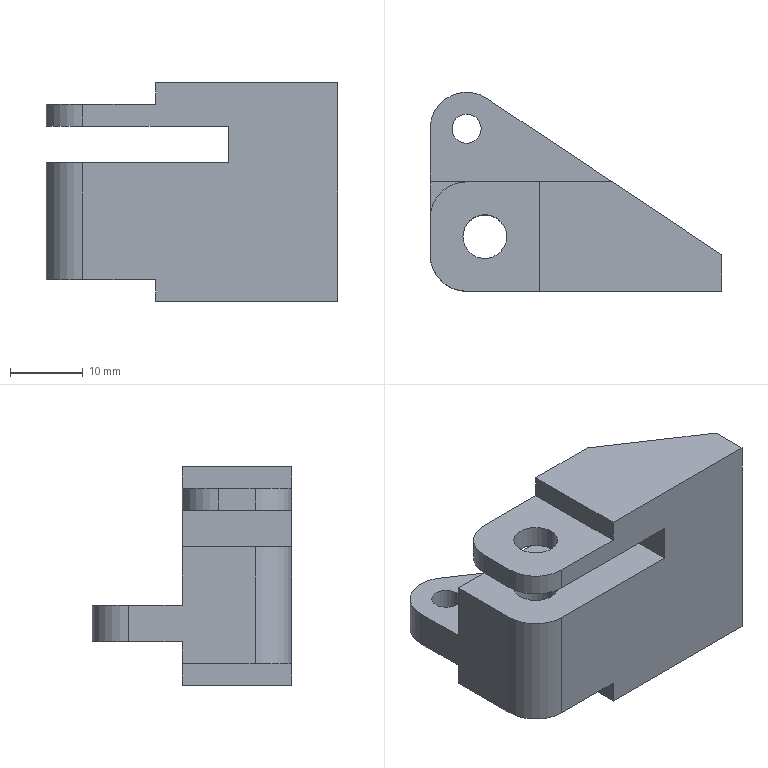Part | SolidWorks | features ICE 4, Fillet 2, Extrusion 1 | 1 solid | 29 faces | box 40 x 27.324 x 30 mm | volume 12750 mm3 | plane 19 | cylinder 10 | commonest cylinder face diameters 6 x4 10 x4 4 x2
STEP:
#1=CARTESIAN_POINT('',(-35.5,7.5,-12.));
#2=VERTEX_POINT('',#1);
#3=CARTESIAN_POINT('',(-29.5,7.5,-12.));
#4=VERTEX_POINT('',#3);
#5=CARTESIAN_POINT('',(-32.5,7.5,-12.));
#6=DIRECTION('',(0.,0.,1.));
#7=DIRECTION('',(1.,0.,0.));
#8=AXIS2_PLACEMENT_3D('',#5,#6,#7);
#9=CIRCLE('',#8,3.);
#10=EDGE_CURVE('',#2,#4,#9,.T.);
#11=ORIENTED_EDGE('',*,*,#10,.F.);
#12=CARTESIAN_POINT('',(-35.5,7.5,4.));
#13=VERTEX_POINT('',#12);
#14=CARTESIAN_POINT('',(-35.5,7.5,-15.));
#15=DIRECTION('',(0.,0.,1.));
#16=VECTOR('',#15,1000.);
#17=LINE('',#14,#16);
#18=EDGE_CURVE('',#2,#13,#17,.T.);
#19=ORIENTED_EDGE('',*,*,#18,.T.);
#20=CARTESIAN_POINT('',(-29.5,7.5,4.));
#21=VERTEX_POINT('',#20);
#22=CARTESIAN_POINT('',(-32.5,7.5,4.));
#23=DIRECTION('',(0.,0.,-1.));
#24=DIRECTION('',(-1.,0.,0.));
#25=AXIS2_PLACEMENT_3D('',#22,#23,#24);
#26=CIRCLE('',#25,3.);
#27=EDGE_CURVE('',#21,#13,#26,.T.);
#28=ORIENTED_EDGE('',*,*,#27,.F.);
#29=CARTESIAN_POINT('',(-29.5,7.5,-15.));
#30=DIRECTION('',(0.,0.,1.));
#31=VECTOR('',#30,1000.);
#32=LINE('',#29,#31);
#33=EDGE_CURVE('',#4,#21,#32,.T.);
#34=ORIENTED_EDGE('',*,*,#33,.F.);
#35=EDGE_LOOP('',(#11,#19,#28,#34));
#36=FACE_OUTER_BOUND('',#35,.T.);
#37=CARTESIAN_POINT('',(-32.5,7.5,-15.));
#38=DIRECTION('',(0.,0.,1.));
#39=DIRECTION('',(1.,0.,0.));
#40=AXIS2_PLACEMENT_3D('',#37,#38,#39);
#41=CYLINDRICAL_SURFACE('',#40,3.);
#42=ADVANCED_FACE('',(#36),#41,.F.);
#43=CARTESIAN_POINT('',(-35.5,7.5,9.));
#44=VERTEX_POINT('',#43);
#45=CARTESIAN_POINT('',(-29.5,7.5,9.));
#46=VERTEX_POINT('',#45);
#47=CARTESIAN_POINT('',(-32.5,7.5,9.));
#48=DIRECTION('',(0.,0.,1.));
#49=DIRECTION('',(1.,0.,0.));
#50=AXIS2_PLACEMENT_3D('',#47,#48,#49);
#51=CIRCLE('',#50,3.);
#52=EDGE_CURVE('',#44,#46,#51,.T.);
#53=ORIENTED_EDGE('',*,*,#52,.F.);
#54=CARTESIAN_POINT('',(-35.5,7.5,12.));
#55=VERTEX_POINT('',#54);
#56=CARTESIAN_POINT('',(-35.5,7.5,-15.));
#57=DIRECTION('',(0.,0.,1.));
#58=VECTOR('',#57,1000.);
#59=LINE('',#56,#58);
#60=EDGE_CURVE('',#44,#55,#59,.T.);
#61=ORIENTED_EDGE('',*,*,#60,.T.);
#62=CARTESIAN_POINT('',(-29.5,7.5,12.));
#63=VERTEX_POINT('',#62);
#64=CARTESIAN_POINT('',(-32.5,7.5,12.));
#65=DIRECTION('',(0.,0.,1.));
#66=DIRECTION('',(1.,0.,0.));
#67=AXIS2_PLACEMENT_3D('',#64,#65,#66);
#68=CIRCLE('',#67,3.);
#69=EDGE_CURVE('',#55,#63,#68,.T.);
#70=ORIENTED_EDGE('',*,*,#69,.T.);
#71=CARTESIAN_POINT('',(-29.5,7.5,-15.));
#72=DIRECTION('',(0.,0.,1.));
#73=VECTOR('',#72,1000.);
#74=LINE('',#71,#73);
#75=EDGE_CURVE('',#46,#63,#74,.T.);
#76=ORIENTED_EDGE('',*,*,#75,.F.);
#77=EDGE_LOOP('',(#53,#61,#70,#76));
#78=FACE_OUTER_BOUND('',#77,.T.);
#79=CARTESIAN_POINT('',(-32.5,7.5,-15.));
#80=DIRECTION('',(0.,0.,1.));
#81=DIRECTION('',(1.,0.,0.));
#82=AXIS2_PLACEMENT_3D('',#79,#80,#81);
#83=CYLINDRICAL_SURFACE('',#82,3.);
#84=ADVANCED_FACE('',(#78),#83,.F.);
#85=CARTESIAN_POINT('',(-37.,22.324,-4.));
#86=VERTEX_POINT('',#85);
#87=CARTESIAN_POINT('',(-33.,22.324,-4.));
#88=VERTEX_POINT('',#87);
#89=CARTESIAN_POINT('',(-35.,22.324,-4.));
#90=DIRECTION('',(0.,0.,1.));
#91=DIRECTION('',(1.,0.,0.));
#92=AXIS2_PLACEMENT_3D('',#89,#90,#91);
#93=CIRCLE('',#92,2.);
#94=EDGE_CURVE('',#86,#88,#93,.T.);
#95=ORIENTED_EDGE('',*,*,#94,.T.);
#96=CARTESIAN_POINT('',(-33.,22.324,-9.));
#97=VERTEX_POINT('',#96);
#98=CARTESIAN_POINT('',(-33.,22.324,-4.));
#99=DIRECTION('',(0.,0.,-1.));
#100=VECTOR('',#99,1000.);
#101=LINE('',#98,#100);
#102=EDGE_CURVE('',#88,#97,#101,.T.);
#103=ORIENTED_EDGE('',*,*,#102,.T.);
#104=CARTESIAN_POINT('',(-37.,22.324,-9.));
#105=VERTEX_POINT('',#104);
#106=CARTESIAN_POINT('',(-35.,22.324,-9.));
#107=DIRECTION('',(0.,0.,1.));
#108=DIRECTION('',(1.,0.,0.));
#109=AXIS2_PLACEMENT_3D('',#106,#107,#108);
#110=CIRCLE('',#109,2.);
#111=EDGE_CURVE('',#105,#97,#110,.T.);
#112=ORIENTED_EDGE('',*,*,#111,.F.);
#113=CARTESIAN_POINT('',(-37.,22.324,-4.));
#114=DIRECTION('',(0.,0.,-1.));
#115=VECTOR('',#114,1000.);
#116=LINE('',#113,#115);
#117=EDGE_CURVE('',#86,#105,#116,.T.);
#118=ORIENTED_EDGE('',*,*,#117,.F.);
#119=EDGE_LOOP('',(#95,#103,#112,#118));
#120=FACE_OUTER_BOUND('',#119,.T.);
#121=CARTESIAN_POINT('',(-35.,22.324,-4.));
#122=DIRECTION('',(0.,0.,-1.));
#123=DIRECTION('',(-1.,0.,0.));
#124=AXIS2_PLACEMENT_3D('',#121,#122,#123);
#125=CYLINDRICAL_SURFACE('',#124,2.);
#126=ADVANCED_FACE('',(#120),#125,.F.);
#127=CARTESIAN_POINT('',(-40.,15.,-9.));
#128=VERTEX_POINT('',#127);
#129=CARTESIAN_POINT('',(-15.,15.,-9.));
#130=VERTEX_POINT('',#129);
#131=CARTESIAN_POINT('',(-40.,15.,-9.));
#132=DIRECTION('',(1.,0.,0.));
#133=VECTOR('',#132,1000.);
#134=LINE('',#131,#133);
#135=EDGE_CURVE('',#128,#130,#134,.T.);
#136=ORIENTED_EDGE('',*,*,#135,.T.);
#137=CARTESIAN_POINT('',(-15.,15.,-15.));
#138=VERTEX_POINT('',#137);
#139=CARTESIAN_POINT('',(-15.,15.,15.));
#140=DIRECTION('',(0.,0.,-1.));
#141=VECTOR('',#140,1000.);
#142=LINE('',#139,#141);
#143=EDGE_CURVE('',#130,#138,#142,.T.);
#144=ORIENTED_EDGE('',*,*,#143,.T.);
#145=CARTESIAN_POINT('',(-25.,15.,-15.));
#146=VERTEX_POINT('',#145);
#147=CARTESIAN_POINT('',(-15.,15.,-15.));
#148=DIRECTION('',(-1.,0.,0.));
#149=VECTOR('',#148,1000.);
#150=LINE('',#147,#149);
#151=EDGE_CURVE('',#138,#146,#150,.T.);
#152=ORIENTED_EDGE('',*,*,#151,.T.);
#153=CARTESIAN_POINT('',(-25.,15.,-12.));
#154=VERTEX_POINT('',#153);
#155=CARTESIAN_POINT('',(-25.,15.,-32.358));
#156=DIRECTION('',(0.,0.,-1.));
#157=VECTOR('',#156,1000.);
#158=LINE('',#155,#157);
#159=EDGE_CURVE('',#154,#146,#158,.T.);
#160=ORIENTED_EDGE('',*,*,#159,.F.);
#161=CARTESIAN_POINT('',(-40.,15.,-12.));
#162=VERTEX_POINT('',#161);
#163=CARTESIAN_POINT('',(-63.199,15.,-12.));
#164=DIRECTION('',(1.,0.,0.));
#165=VECTOR('',#164,1000.);
#166=LINE('',#163,#165);
#167=EDGE_CURVE('',#162,#154,#166,.T.);
#168=ORIENTED_EDGE('',*,*,#167,.F.);
#169=CARTESIAN_POINT('',(-40.,15.,15.));
#170=DIRECTION('',(0.,0.,-1.));
#171=VECTOR('',#170,1000.);
#172=LINE('',#169,#171);
#173=EDGE_CURVE('',#128,#162,#172,.T.);
#174=ORIENTED_EDGE('',*,*,#173,.F.);
#175=EDGE_LOOP('',(#136,#144,#152,#160,#168,#174));
#176=FACE_OUTER_BOUND('',#175,.T.);
#177=CARTESIAN_POINT('',(-15.,15.,15.));
#178=DIRECTION('',(0.,-1.,0.));
#179=DIRECTION('',(0.,0.,-1.));
#180=AXIS2_PLACEMENT_3D('',#177,#178,#179);
#181=PLANE('',#180);
#182=ADVANCED_FACE('',(#176),#181,.F.);
#183=CARTESIAN_POINT('',(-15.,15.,4.));
#184=VERTEX_POINT('',#183);
#185=CARTESIAN_POINT('',(-15.,15.,-4.));
#186=VERTEX_POINT('',#185);
#187=CARTESIAN_POINT('',(-15.,15.,15.));
#188=DIRECTION('',(0.,0.,-1.));
#189=VECTOR('',#188,1000.);
#190=LINE('',#187,#189);
#191=EDGE_CURVE('',#184,#186,#190,.T.);
#192=ORIENTED_EDGE('',*,*,#191,.T.);
#193=CARTESIAN_POINT('',(-40.,15.,-4.));
#194=VERTEX_POINT('',#193);
#195=CARTESIAN_POINT('',(-40.,15.,-4.));
#196=DIRECTION('',(1.,0.,0.));
#197=VECTOR('',#196,1000.);
#198=LINE('',#195,#197);
#199=EDGE_CURVE('',#194,#186,#198,.T.);
#200=ORIENTED_EDGE('',*,*,#199,.F.);
#201=CARTESIAN_POINT('',(-40.,15.,4.));
#202=VERTEX_POINT('',#201);
#203=CARTESIAN_POINT('',(-40.,15.,15.));
#204=DIRECTION('',(0.,0.,-1.));
#205=VECTOR('',#204,1000.);
#206=LINE('',#203,#205);
#207=EDGE_CURVE('',#202,#194,#206,.T.);
#208=ORIENTED_EDGE('',*,*,#207,.F.);
#209=CARTESIAN_POINT('',(-40.,15.,4.));
#210=DIRECTION('',(-1.,0.,0.));
#211=VECTOR('',#210,1000.);
#212=LINE('',#209,#211);
#213=EDGE_CURVE('',#184,#202,#212,.T.);
#214=ORIENTED_EDGE('',*,*,#213,.F.);
#215=EDGE_LOOP('',(#192,#200,#208,#214));
#216=FACE_OUTER_BOUND('',#215,.T.);
#217=CARTESIAN_POINT('',(-15.,15.,15.));
#218=DIRECTION('',(0.,-1.,0.));
#219=DIRECTION('',(0.,0.,-1.));
#220=AXIS2_PLACEMENT_3D('',#217,#218,#219);
#221=PLANE('',#220);
#222=ADVANCED_FACE('',(#216),#221,.F.);
#223=CARTESIAN_POINT('',(-40.,5.,-12.));
#224=VERTEX_POINT('',#223);
#225=CARTESIAN_POINT('',(-40.,15.,-12.));
#226=DIRECTION('',(0.,-1.,0.));
#227=VECTOR('',#226,1000.);
#228=LINE('',#225,#227);
#229=EDGE_CURVE('',#162,#224,#228,.T.);
#230=ORIENTED_EDGE('',*,*,#229,.T.);
#231=CARTESIAN_POINT('',(-40.,5.,4.));
#232=VERTEX_POINT('',#231);
#233=CARTESIAN_POINT('',(-40.,5.,15.));
#234=DIRECTION('',(0.,0.,1.));
#235=VECTOR('',#234,1000.);
#236=LINE('',#233,#235);
#237=EDGE_CURVE('',#224,#232,#236,.T.);
#238=ORIENTED_EDGE('',*,*,#237,.T.);
#239=CARTESIAN_POINT('',(-40.,15.,4.));
#240=DIRECTION('',(0.,1.,0.));
#241=VECTOR('',#240,1000.);
#242=LINE('',#239,#241);
#243=EDGE_CURVE('',#232,#202,#242,.T.);
#244=ORIENTED_EDGE('',*,*,#243,.T.);
#245=ORIENTED_EDGE('',*,*,#207,.T.);
#246=CARTESIAN_POINT('',(-40.,22.324,-4.));
#247=VERTEX_POINT('',#246);
#248=CARTESIAN_POINT('',(-40.,15.,-4.));
#249=DIRECTION('',(0.,-1.,0.));
#250=VECTOR('',#249,1000.);
#251=LINE('',#248,#250);
#252=EDGE_CURVE('',#247,#194,#251,.T.);
#253=ORIENTED_EDGE('',*,*,#252,.F.);
#254=CARTESIAN_POINT('',(-40.,22.324,-9.));
#255=VERTEX_POINT('',#254);
#256=CARTESIAN_POINT('',(-40.,22.324,-4.));
#257=DIRECTION('',(0.,0.,-1.));
#258=VECTOR('',#257,1000.);
#259=LINE('',#256,#258);
#260=EDGE_CURVE('',#247,#255,#259,.T.);
#261=ORIENTED_EDGE('',*,*,#260,.T.);
#262=CARTESIAN_POINT('',(-40.,15.,-9.));
#263=DIRECTION('',(0.,-1.,0.));
#264=VECTOR('',#263,1000.);
#265=LINE('',#262,#264);
#266=EDGE_CURVE('',#255,#128,#265,.T.);
#267=ORIENTED_EDGE('',*,*,#266,.T.);
#268=ORIENTED_EDGE('',*,*,#173,.T.);
#269=EDGE_LOOP('',(#230,#238,#244,#245,#253,#261,#267,#268));
#270=FACE_OUTER_BOUND('',#269,.T.);
#271=CARTESIAN_POINT('',(-40.,15.,15.));
#272=DIRECTION('',(1.,0.,0.));
#273=DIRECTION('',(0.,0.,-1.));
#274=AXIS2_PLACEMENT_3D('',#271,#272,#273);
#275=PLANE('',#274);
#276=ADVANCED_FACE('',(#270),#275,.F.);
#277=CARTESIAN_POINT('',(-15.,0.,4.));
#278=VERTEX_POINT('',#277);
#279=CARTESIAN_POINT('',(-35.,0.,4.));
#280=VERTEX_POINT('',#279);
#281=CARTESIAN_POINT('',(-40.,0.,4.));
#282=DIRECTION('',(-1.,0.,0.));
#283=VECTOR('',#282,1000.);
#284=LINE('',#281,#283);
#285=EDGE_CURVE('',#278,#280,#284,.T.);
#286=ORIENTED_EDGE('',*,*,#285,.T.);
#287=CARTESIAN_POINT('',(-35.,0.,-12.));
#288=VERTEX_POINT('',#287);
#289=CARTESIAN_POINT('',(-35.,0.,15.));
#290=DIRECTION('',(0.,0.,-1.));
#291=VECTOR('',#290,1000.);
#292=LINE('',#289,#291);
#293=EDGE_CURVE('',#280,#288,#292,.T.);
#294=ORIENTED_EDGE('',*,*,#293,.T.);
#295=CARTESIAN_POINT('',(-25.,0.,-12.));
#296=VERTEX_POINT('',#295);
#297=CARTESIAN_POINT('',(-40.,0.,-12.));
#298=DIRECTION('',(1.,0.,0.));
#299=VECTOR('',#298,1000.);
#300=LINE('',#297,#299);
#301=EDGE_CURVE('',#288,#296,#300,.T.);
#302=ORIENTED_EDGE('',*,*,#301,.T.);
#303=CARTESIAN_POINT('',(-25.,0.,-15.));
#304=VERTEX_POINT('',#303);
#305=CARTESIAN_POINT('',(-25.,0.,15.));
#306=DIRECTION('',(0.,0.,-1.));
#307=VECTOR('',#306,1000.);
#308=LINE('',#305,#307);
#309=EDGE_CURVE('',#296,#304,#308,.T.);
#310=ORIENTED_EDGE('',*,*,#309,.T.);
#311=CARTESIAN_POINT('',(0.,0.,-15.));
#312=VERTEX_POINT('',#311);
#313=CARTESIAN_POINT('',(-40.,0.,-15.));
#314=DIRECTION('',(1.,0.,0.));
#315=VECTOR('',#314,1000.);
#316=LINE('',#313,#315);
#317=EDGE_CURVE('',#304,#312,#316,.T.);
#318=ORIENTED_EDGE('',*,*,#317,.T.);
#319=CARTESIAN_POINT('',(0.,0.,15.));
#320=VERTEX_POINT('',#319);
#321=CARTESIAN_POINT('',(0.,0.,15.));
#322=DIRECTION('',(0.,0.,-1.));
#323=VECTOR('',#322,1000.);
#324=LINE('',#321,#323);
#325=EDGE_CURVE('',#320,#312,#324,.T.);
#326=ORIENTED_EDGE('',*,*,#325,.F.);
#327=CARTESIAN_POINT('',(-25.,0.,15.));
#328=VERTEX_POINT('',#327);
#329=CARTESIAN_POINT('',(-40.,0.,15.));
#330=DIRECTION('',(1.,0.,0.));
#331=VECTOR('',#330,1000.);
#332=LINE('',#329,#331);
#333=EDGE_CURVE('',#328,#320,#332,.T.);
#334=ORIENTED_EDGE('',*,*,#333,.F.);
#335=CARTESIAN_POINT('',(-25.,0.,12.));
#336=VERTEX_POINT('',#335);
#337=CARTESIAN_POINT('',(-25.,0.,15.));
#338=DIRECTION('',(0.,0.,-1.));
#339=VECTOR('',#338,1000.);
#340=LINE('',#337,#339);
#341=EDGE_CURVE('',#328,#336,#340,.T.);
#342=ORIENTED_EDGE('',*,*,#341,.T.);
#343=CARTESIAN_POINT('',(-35.,0.,12.));
#344=VERTEX_POINT('',#343);
#345=CARTESIAN_POINT('',(-40.,0.,12.));
#346=DIRECTION('',(-1.,0.,0.));
#347=VECTOR('',#346,1000.);
#348=LINE('',#345,#347);
#349=EDGE_CURVE('',#336,#344,#348,.T.);
#350=ORIENTED_EDGE('',*,*,#349,.T.);
#351=CARTESIAN_POINT('',(-35.,0.,9.));
#352=VERTEX_POINT('',#351);
#353=CARTESIAN_POINT('',(-35.,0.,15.));
#354=DIRECTION('',(0.,0.,-1.));
#355=VECTOR('',#354,1000.);
#356=LINE('',#353,#355);
#357=EDGE_CURVE('',#344,#352,#356,.T.);
#358=ORIENTED_EDGE('',*,*,#357,.T.);
#359=CARTESIAN_POINT('',(-15.,0.,9.));
#360=VERTEX_POINT('',#359);
#361=CARTESIAN_POINT('',(-40.,0.,9.));
#362=DIRECTION('',(1.,0.,0.));
#363=VECTOR('',#362,1000.);
#364=LINE('',#361,#363);
#365=EDGE_CURVE('',#352,#360,#364,.T.);
#366=ORIENTED_EDGE('',*,*,#365,.T.);
#367=CARTESIAN_POINT('',(-15.,0.,15.));
#368=DIRECTION('',(0.,0.,-1.));
#369=VECTOR('',#368,1000.);
#370=LINE('',#367,#369);
#371=EDGE_CURVE('',#360,#278,#370,.T.);
#372=ORIENTED_EDGE('',*,*,#371,.T.);
#373=EDGE_LOOP('',(#286,#294,#302,#310,#318,#326,#334,#342,#350,#358,#366,#372));
#374=FACE_OUTER_BOUND('',#373,.T.);
#375=CARTESIAN_POINT('',(-40.,0.,15.));
#376=DIRECTION('',(0.,1.,0.));
#377=DIRECTION('',(0.,0.,1.));
#378=AXIS2_PLACEMENT_3D('',#375,#376,#377);
#379=PLANE('',#378);
#380=ADVANCED_FACE('',(#374),#379,.F.);
#381=CARTESIAN_POINT('',(0.,5.,-15.));
#382=VERTEX_POINT('',#381);
#383=CARTESIAN_POINT('',(0.,0.,-15.));
#384=DIRECTION('',(0.,1.,0.));
#385=VECTOR('',#384,1000.);
#386=LINE('',#383,#385);
#387=EDGE_CURVE('',#312,#382,#386,.T.);
#388=ORIENTED_EDGE('',*,*,#387,.T.);
#389=CARTESIAN_POINT('',(0.,5.,15.));
#390=VERTEX_POINT('',#389);
#391=CARTESIAN_POINT('',(0.,5.,15.));
#392=DIRECTION('',(0.,0.,-1.));
#393=VECTOR('',#392,1000.);
#394=LINE('',#391,#393);
#395=EDGE_CURVE('',#390,#382,#394,.T.);
#396=ORIENTED_EDGE('',*,*,#395,.F.);
#397=CARTESIAN_POINT('',(0.,0.,15.));
#398=DIRECTION('',(0.,1.,0.));
#399=VECTOR('',#398,1000.);
#400=LINE('',#397,#399);
#401=EDGE_CURVE('',#320,#390,#400,.T.);
#402=ORIENTED_EDGE('',*,*,#401,.F.);
#403=ORIENTED_EDGE('',*,*,#325,.T.);
#404=EDGE_LOOP('',(#388,#396,#402,#403));
#405=FACE_OUTER_BOUND('',#404,.T.);
#406=CARTESIAN_POINT('',(0.,0.,15.));
#407=DIRECTION('',(-1.,0.,0.));
#408=DIRECTION('',(0.,0.,1.));
#409=AXIS2_PLACEMENT_3D('',#406,#407,#408);
#410=PLANE('',#409);
#411=ADVANCED_FACE('',(#405),#410,.F.);
#412=CARTESIAN_POINT('',(0.,5.,-15.));
#413=DIRECTION('',(-0.8321,0.5547,0.));
#414=VECTOR('',#413,1000.);
#415=LINE('',#412,#414);
#416=EDGE_CURVE('',#382,#138,#415,.T.);
#417=ORIENTED_EDGE('',*,*,#416,.T.);
#418=ORIENTED_EDGE('',*,*,#143,.F.);
#419=CARTESIAN_POINT('',(-32.226,26.484,-9.));
#420=VERTEX_POINT('',#419);
#421=CARTESIAN_POINT('',(-15.,15.,-9.));
#422=DIRECTION('',(-0.8321,0.5547,0.));
#423=VECTOR('',#422,1000.);
#424=LINE('',#421,#423);
#425=EDGE_CURVE('',#130,#420,#424,.T.);
#426=ORIENTED_EDGE('',*,*,#425,.T.);
#427=CARTESIAN_POINT('',(-32.226,26.484,-4.));
#428=VERTEX_POINT('',#427);
#429=CARTESIAN_POINT('',(-32.226,26.484,-4.));
#430=DIRECTION('',(0.,0.,-1.));
#431=VECTOR('',#430,1000.);
#432=LINE('',#429,#431);
#433=EDGE_CURVE('',#428,#420,#432,.T.);
#434=ORIENTED_EDGE('',*,*,#433,.F.);
#435=CARTESIAN_POINT('',(-15.,15.,-4.));
#436=DIRECTION('',(-0.8321,0.5547,0.));
#437=VECTOR('',#436,1000.);
#438=LINE('',#435,#437);
#439=EDGE_CURVE('',#186,#428,#438,.T.);
#440=ORIENTED_EDGE('',*,*,#439,.F.);
#441=ORIENTED_EDGE('',*,*,#191,.F.);
#442=CARTESIAN_POINT('',(-15.,15.,9.));
#443=VERTEX_POINT('',#442);
#444=CARTESIAN_POINT('',(-15.,15.,4.));
#445=DIRECTION('',(0.,0.,-1.));
#446=VECTOR('',#445,1000.);
#447=LINE('',#444,#446);
#448=EDGE_CURVE('',#443,#184,#447,.T.);
#449=ORIENTED_EDGE('',*,*,#448,.F.);
#450=CARTESIAN_POINT('',(-15.,15.,15.));
#451=VERTEX_POINT('',#450);
#452=CARTESIAN_POINT('',(-15.,15.,15.));
#453=DIRECTION('',(0.,0.,-1.));
#454=VECTOR('',#453,1000.);
#455=LINE('',#452,#454);
#456=EDGE_CURVE('',#451,#443,#455,.T.);
#457=ORIENTED_EDGE('',*,*,#456,.F.);
#458=CARTESIAN_POINT('',(0.,5.,15.));
#459=DIRECTION('',(-0.8321,0.5547,0.));
#460=VECTOR('',#459,1000.);
#461=LINE('',#458,#460);
#462=EDGE_CURVE('',#390,#451,#461,.T.);
#463=ORIENTED_EDGE('',*,*,#462,.F.);
#464=ORIENTED_EDGE('',*,*,#395,.T.);
#465=EDGE_LOOP('',(#417,#418,#426,#434,#440,#441,#449,#457,#463,#464));
#466=FACE_OUTER_BOUND('',#465,.T.);
#467=CARTESIAN_POINT('',(0.,5.,15.));
#468=DIRECTION('',(-0.5547,-0.8321,0.));
#469=DIRECTION('',(0.8321,-0.5547,0.));
#470=AXIS2_PLACEMENT_3D('',#467,#468,#469);
#471=PLANE('',#470);
#472=ADVANCED_FACE('',(#466),#471,.F.);
#473=CARTESIAN_POINT('',(-35.,15.,9.));
#474=VERTEX_POINT('',#473);
#475=CARTESIAN_POINT('',(-40.,15.,9.));
#476=DIRECTION('',(1.,0.,0.));
#477=VECTOR('',#476,1000.);
#478=LINE('',#475,#477);
#479=EDGE_CURVE('',#474,#443,#478,.T.);
#480=ORIENTED_EDGE('',*,*,#479,.F.);
#481=CARTESIAN_POINT('',(-35.,15.,12.));
#482=VERTEX_POINT('',#481);
#483=CARTESIAN_POINT('',(-35.,15.,15.));
#484=DIRECTION('',(0.,0.,1.));
#485=VECTOR('',#484,1000.);
#486=LINE('',#483,#485);
#487=EDGE_CURVE('',#474,#482,#486,.T.);
#488=ORIENTED_EDGE('',*,*,#487,.T.);
#489=CARTESIAN_POINT('',(-25.,15.,12.));
#490=VERTEX_POINT('',#489);
#491=CARTESIAN_POINT('',(-63.199,15.,12.));
#492=DIRECTION('',(-1.,0.,0.));
#493=VECTOR('',#492,1000.);
#494=LINE('',#491,#493);
#495=EDGE_CURVE('',#490,#482,#494,.T.);
#496=ORIENTED_EDGE('',*,*,#495,.F.);
#497=CARTESIAN_POINT('',(-25.,15.,15.));
#498=VERTEX_POINT('',#497);
#499=CARTESIAN_POINT('',(-25.,15.,32.358));
#500=DIRECTION('',(0.,0.,-1.));
#501=VECTOR('',#500,1000.);
#502=LINE('',#499,#501);
#503=EDGE_CURVE('',#498,#490,#502,.T.);
#504=ORIENTED_EDGE('',*,*,#503,.F.);
#505=CARTESIAN_POINT('',(-15.,15.,15.));
#506=DIRECTION('',(-1.,0.,0.));
#507=VECTOR('',#506,1000.);
#508=LINE('',#505,#507);
#509=EDGE_CURVE('',#451,#498,#508,.T.);
#510=ORIENTED_EDGE('',*,*,#509,.F.);
#511=ORIENTED_EDGE('',*,*,#456,.T.);
#512=EDGE_LOOP('',(#480,#488,#496,#504,#510,#511));
#513=FACE_OUTER_BOUND('',#512,.T.);
#514=CARTESIAN_POINT('',(-15.,15.,15.));
#515=DIRECTION('',(0.,-1.,0.));
#516=DIRECTION('',(0.,0.,-1.));
#517=AXIS2_PLACEMENT_3D('',#514,#515,#516);
#518=PLANE('',#517);
#519=ADVANCED_FACE('',(#513),#518,.F.);
#520=CARTESIAN_POINT('',(-40.,5.,12.));
#521=VERTEX_POINT('',#520);
#522=CARTESIAN_POINT('',(-40.,10.,12.));
#523=VERTEX_POINT('',#522);
#524=CARTESIAN_POINT('',(-40.,15.,12.));
#525=DIRECTION('',(0.,1.,0.));
#526=VECTOR('',#525,1000.);
#527=LINE('',#524,#526);
#528=EDGE_CURVE('',#521,#523,#527,.T.);
#529=ORIENTED_EDGE('',*,*,#528,.T.);
#530=CARTESIAN_POINT('',(-40.,10.,9.));
#531=VERTEX_POINT('',#530);
#532=CARTESIAN_POINT('',(-40.,10.,15.));
#533=DIRECTION('',(0.,0.,-1.));
#534=VECTOR('',#533,1000.);
#535=LINE('',#532,#534);
#536=EDGE_CURVE('',#523,#531,#535,.T.);
#537=ORIENTED_EDGE('',*,*,#536,.T.);
#538=CARTESIAN_POINT('',(-40.,5.,9.));
#539=VERTEX_POINT('',#538);
#540=CARTESIAN_POINT('',(-40.,15.,9.));
#541=DIRECTION('',(0.,-1.,0.));
#542=VECTOR('',#541,1000.);
#543=LINE('',#540,#542);
#544=EDGE_CURVE('',#531,#539,#543,.T.);
#545=ORIENTED_EDGE('',*,*,#544,.T.);
#546=CARTESIAN_POINT('',(-40.,5.,15.));
#547=DIRECTION('',(0.,0.,1.));
#548=VECTOR('',#547,1000.);
#549=LINE('',#546,#548);
#550=EDGE_CURVE('',#539,#521,#549,.T.);
#551=ORIENTED_EDGE('',*,*,#550,.T.);
#552=EDGE_LOOP('',(#529,#537,#545,#551));
#553=FACE_OUTER_BOUND('',#552,.T.);
#554=CARTESIAN_POINT('',(-40.,15.,15.));
#555=DIRECTION('',(1.,0.,0.));
#556=DIRECTION('',(0.,0.,-1.));
#557=AXIS2_PLACEMENT_3D('',#554,#555,#556);
#558=PLANE('',#557);
#559=ADVANCED_FACE('',(#553),#558,.F.);
#560=CARTESIAN_POINT('',(-25.,0.,15.));
#561=DIRECTION('',(0.,1.,0.));
#562=VECTOR('',#561,1000.);
#563=LINE('',#560,#562);
#564=EDGE_CURVE('',#328,#498,#563,.T.);
#565=ORIENTED_EDGE('',*,*,#564,.F.);
#566=ORIENTED_EDGE('',*,*,#333,.T.);
#567=ORIENTED_EDGE('',*,*,#401,.T.);
#568=ORIENTED_EDGE('',*,*,#462,.T.);
#569=ORIENTED_EDGE('',*,*,#509,.T.);
#570=EDGE_LOOP('',(#565,#566,#567,#568,#569));
#571=FACE_OUTER_BOUND('',#570,.T.);
#572=CARTESIAN_POINT('',(0.,0.,15.));
#573=DIRECTION('',(0.,0.,1.));
#574=DIRECTION('',(1.,0.,0.));
#575=AXIS2_PLACEMENT_3D('',#572,#573,#574);
#576=PLANE('',#575);
#577=ADVANCED_FACE('',(#571),#576,.T.);
#578=ORIENTED_EDGE('',*,*,#317,.F.);
#579=CARTESIAN_POINT('',(-25.,0.,-15.));
#580=DIRECTION('',(0.,1.,0.));
#581=VECTOR('',#580,1000.);
#582=LINE('',#579,#581);
#583=EDGE_CURVE('',#304,#146,#582,.T.);
#584=ORIENTED_EDGE('',*,*,#583,.T.);
#585=ORIENTED_EDGE('',*,*,#151,.F.);
#586=ORIENTED_EDGE('',*,*,#416,.F.);
#587=ORIENTED_EDGE('',*,*,#387,.F.);
#588=EDGE_LOOP('',(#578,#584,#585,#586,#587));
#589=FACE_OUTER_BOUND('',#588,.T.);
#590=CARTESIAN_POINT('',(0.,0.,-15.));
#591=DIRECTION('',(0.,0.,1.));
#592=DIRECTION('',(1.,0.,0.));
#593=AXIS2_PLACEMENT_3D('',#590,#591,#592);
#594=PLANE('',#593);
#595=ADVANCED_FACE('',(#589),#594,.F.);
#596=CARTESIAN_POINT('',(-32.5,7.5,-12.));
#597=DIRECTION('',(0.,0.,1.));
#598=DIRECTION('',(1.,0.,0.));
#599=AXIS2_PLACEMENT_3D('',#596,#597,#598);
#600=CIRCLE('',#599,3.);
#601=EDGE_CURVE('',#4,#2,#600,.T.);
#602=ORIENTED_EDGE('',*,*,#601,.T.);
#603=ORIENTED_EDGE('',*,*,#10,.T.);
#604=EDGE_LOOP('',(#602,#603));
#605=FACE_BOUND('',#604,.T.);
#606=ORIENTED_EDGE('',*,*,#301,.F.);
#607=CARTESIAN_POINT('',(-35.,5.,-12.));
#608=DIRECTION('',(0.,0.,-1.));
#609=DIRECTION('',(1.,0.,0.));
#610=AXIS2_PLACEMENT_3D('',#607,#608,#609);
#611=CIRCLE('',#610,5.);
#612=EDGE_CURVE('',#288,#224,#611,.T.);
#613=ORIENTED_EDGE('',*,*,#612,.T.);
#614=ORIENTED_EDGE('',*,*,#229,.F.);
#615=ORIENTED_EDGE('',*,*,#167,.T.);
#616=CARTESIAN_POINT('',(-25.,-15.,-12.));
#617=DIRECTION('',(0.,1.,0.));
#618=VECTOR('',#617,1000.);
#619=LINE('',#616,#618);
#620=EDGE_CURVE('',#296,#154,#619,.T.);
#621=ORIENTED_EDGE('',*,*,#620,.F.);
#622=EDGE_LOOP('',(#606,#613,#614,#615,#621));
#623=FACE_OUTER_BOUND('',#622,.T.);
#624=CARTESIAN_POINT('',(-63.199,-15.,-12.));
#625=DIRECTION('',(0.,0.,1.));
#626=DIRECTION('',(1.,0.,0.));
#627=AXIS2_PLACEMENT_3D('',#624,#625,#626);
#628=PLANE('',#627);
#629=ADVANCED_FACE('',(#605,#623),#628,.F.);
#630=ORIENTED_EDGE('',*,*,#620,.T.);
#631=ORIENTED_EDGE('',*,*,#159,.T.);
#632=ORIENTED_EDGE('',*,*,#583,.F.);
#633=ORIENTED_EDGE('',*,*,#309,.F.);
#634=EDGE_LOOP('',(#630,#631,#632,#633));
#635=FACE_OUTER_BOUND('',#634,.T.);
#636=CARTESIAN_POINT('',(-25.,-15.,-32.358));
#637=DIRECTION('',(1.,0.,0.));
#638=DIRECTION('',(0.,0.,-1.));
#639=AXIS2_PLACEMENT_3D('',#636,#637,#638);
#640=PLANE('',#639);
#641=ADVANCED_FACE('',(#635),#640,.F.);
#642=CARTESIAN_POINT('',(-32.5,7.5,12.));
#643=DIRECTION('',(0.,0.,1.));
#644=DIRECTION('',(1.,0.,0.));
#645=AXIS2_PLACEMENT_3D('',#642,#643,#644);
#646=CIRCLE('',#645,3.);
#647=EDGE_CURVE('',#63,#55,#646,.T.);
#648=ORIENTED_EDGE('',*,*,#647,.F.);
#649=ORIENTED_EDGE('',*,*,#69,.F.);
#650=EDGE_LOOP('',(#648,#649));
#651=FACE_BOUND('',#650,.T.);
#652=ORIENTED_EDGE('',*,*,#495,.T.);
#653=CARTESIAN_POINT('',(-35.,10.,12.));
#654=DIRECTION('',(0.,0.,1.));
#655=DIRECTION('',(-1.,0.,0.));
#656=AXIS2_PLACEMENT_3D('',#653,#654,#655);
#657=CIRCLE('',#656,5.);
#658=EDGE_CURVE('',#482,#523,#657,.T.);
#659=ORIENTED_EDGE('',*,*,#658,.T.);
#660=ORIENTED_EDGE('',*,*,#528,.F.);
#661=CARTESIAN_POINT('',(-35.,5.,12.));
#662=DIRECTION('',(0.,0.,1.));
#663=DIRECTION('',(-1.,0.,0.));
#664=AXIS2_PLACEMENT_3D('',#661,#662,#663);
#665=CIRCLE('',#664,5.);
#666=EDGE_CURVE('',#521,#344,#665,.T.);
#667=ORIENTED_EDGE('',*,*,#666,.T.);
#668=ORIENTED_EDGE('',*,*,#349,.F.);
#669=CARTESIAN_POINT('',(-25.,-15.,12.));
#670=DIRECTION('',(0.,1.,0.));
#671=VECTOR('',#670,1000.);
#672=LINE('',#669,#671);
#673=EDGE_CURVE('',#336,#490,#672,.T.);
#674=ORIENTED_EDGE('',*,*,#673,.T.);
#675=EDGE_LOOP('',(#652,#659,#660,#667,#668,#674));
#676=FACE_OUTER_BOUND('',#675,.T.);
#677=CARTESIAN_POINT('',(-63.199,-15.,12.));
#678=DIRECTION('',(0.,0.,-1.));
#679=DIRECTION('',(-1.,0.,0.));
#680=AXIS2_PLACEMENT_3D('',#677,#678,#679);
#681=PLANE('',#680);
#682=ADVANCED_FACE('',(#651,#676),#681,.F.);
#683=ORIENTED_EDGE('',*,*,#564,.T.);
#684=ORIENTED_EDGE('',*,*,#503,.T.);
#685=ORIENTED_EDGE('',*,*,#673,.F.);
#686=ORIENTED_EDGE('',*,*,#341,.F.);
#687=EDGE_LOOP('',(#683,#684,#685,#686));
#688=FACE_OUTER_BOUND('',#687,.T.);
#689=CARTESIAN_POINT('',(-25.,-15.,32.358));
#690=DIRECTION('',(1.,0.,0.));
#691=DIRECTION('',(0.,0.,-1.));
#692=AXIS2_PLACEMENT_3D('',#689,#690,#691);
#693=PLANE('',#692);
#694=ADVANCED_FACE('',(#688),#693,.F.);
#695=CARTESIAN_POINT('',(-15.,-15.,9.));
#696=DIRECTION('',(0.,1.,0.));
#697=VECTOR('',#696,1000.);
#698=LINE('',#695,#697);
#699=EDGE_CURVE('',#360,#443,#698,.T.);
#700=ORIENTED_EDGE('',*,*,#699,.T.);
#701=ORIENTED_EDGE('',*,*,#448,.T.);
#702=CARTESIAN_POINT('',(-15.,-15.,4.));
#703=DIRECTION('',(0.,1.,0.));
#704=VECTOR('',#703,1000.);
#705=LINE('',#702,#704);
#706=EDGE_CURVE('',#278,#184,#705,.T.);
#707=ORIENTED_EDGE('',*,*,#706,.F.);
#708=ORIENTED_EDGE('',*,*,#371,.F.);
#709=EDGE_LOOP('',(#700,#701,#707,#708));
#710=FACE_OUTER_BOUND('',#709,.T.);
#711=CARTESIAN_POINT('',(-15.,-15.,4.));
#712=DIRECTION('',(1.,0.,0.));
#713=DIRECTION('',(0.,0.,-1.));
#714=AXIS2_PLACEMENT_3D('',#711,#712,#713);
#715=PLANE('',#714);
#716=ADVANCED_FACE('',(#710),#715,.F.);
#717=ORIENTED_EDGE('',*,*,#27,.T.);
#718=CARTESIAN_POINT('',(-32.5,7.5,4.));
#719=DIRECTION('',(0.,0.,-1.));
#720=DIRECTION('',(-1.,0.,0.));
#721=AXIS2_PLACEMENT_3D('',#718,#719,#720);
#722=CIRCLE('',#721,3.);
#723=EDGE_CURVE('',#13,#21,#722,.T.);
#724=ORIENTED_EDGE('',*,*,#723,.T.);
#725=EDGE_LOOP('',(#717,#724));
#726=FACE_BOUND('',#725,.T.);
#727=ORIENTED_EDGE('',*,*,#243,.F.);
#728=CARTESIAN_POINT('',(-35.,5.,4.));
#729=DIRECTION('',(0.,0.,1.));
#730=DIRECTION('',(-1.,0.,0.));
#731=AXIS2_PLACEMENT_3D('',#728,#729,#730);
#732=CIRCLE('',#731,5.);
#733=EDGE_CURVE('',#232,#280,#732,.T.);
#734=ORIENTED_EDGE('',*,*,#733,.T.);
#735=ORIENTED_EDGE('',*,*,#285,.F.);
#736=ORIENTED_EDGE('',*,*,#706,.T.);
#737=ORIENTED_EDGE('',*,*,#213,.T.);
#738=EDGE_LOOP('',(#727,#734,#735,#736,#737));
#739=FACE_OUTER_BOUND('',#738,.T.);
#740=CARTESIAN_POINT('',(-40.,-15.,4.));
#741=DIRECTION('',(0.,0.,-1.));
#742=DIRECTION('',(-1.,0.,0.));
#743=AXIS2_PLACEMENT_3D('',#740,#741,#742);
#744=PLANE('',#743);
#745=ADVANCED_FACE('',(#726,#739),#744,.F.);
#746=CARTESIAN_POINT('',(-32.5,7.5,9.));
#747=DIRECTION('',(0.,0.,1.));
#748=DIRECTION('',(1.,0.,0.));
#749=AXIS2_PLACEMENT_3D('',#746,#747,#748);
#750=CIRCLE('',#749,3.);
#751=EDGE_CURVE('',#46,#44,#750,.T.);
#752=ORIENTED_EDGE('',*,*,#751,.T.);
#753=ORIENTED_EDGE('',*,*,#52,.T.);
#754=EDGE_LOOP('',(#752,#753));
#755=FACE_BOUND('',#754,.T.);
#756=ORIENTED_EDGE('',*,*,#544,.F.);
#757=CARTESIAN_POINT('',(-35.,10.,9.));
#758=DIRECTION('',(0.,0.,-1.));
#759=DIRECTION('',(1.,0.,0.));
#760=AXIS2_PLACEMENT_3D('',#757,#758,#759);
#761=CIRCLE('',#760,5.);
#762=EDGE_CURVE('',#531,#474,#761,.T.);
#763=ORIENTED_EDGE('',*,*,#762,.T.);
#764=ORIENTED_EDGE('',*,*,#479,.T.);
#765=ORIENTED_EDGE('',*,*,#699,.F.);
#766=ORIENTED_EDGE('',*,*,#365,.F.);
#767=CARTESIAN_POINT('',(-35.,5.,9.));
#768=DIRECTION('',(0.,0.,-1.));
#769=DIRECTION('',(1.,0.,0.));
#770=AXIS2_PLACEMENT_3D('',#767,#768,#769);
#771=CIRCLE('',#770,5.);
#772=EDGE_CURVE('',#352,#539,#771,.T.);
#773=ORIENTED_EDGE('',*,*,#772,.T.);
#774=EDGE_LOOP('',(#756,#763,#764,#765,#766,#773));
#775=FACE_OUTER_BOUND('',#774,.T.);
#776=CARTESIAN_POINT('',(-40.,-15.,9.));
#777=DIRECTION('',(0.,0.,1.));
#778=DIRECTION('',(1.,0.,0.));
#779=AXIS2_PLACEMENT_3D('',#776,#777,#778);
#780=PLANE('',#779);
#781=ADVANCED_FACE('',(#755,#775),#780,.F.);
#782=ORIENTED_EDGE('',*,*,#199,.T.);
#783=ORIENTED_EDGE('',*,*,#439,.T.);
#784=CARTESIAN_POINT('',(-35.,22.324,-4.));
#785=DIRECTION('',(0.,0.,1.));
#786=DIRECTION('',(1.,0.,0.));
#787=AXIS2_PLACEMENT_3D('',#784,#785,#786);
#788=CIRCLE('',#787,5.);
#789=EDGE_CURVE('',#428,#247,#788,.T.);
#790=ORIENTED_EDGE('',*,*,#789,.T.);
#791=ORIENTED_EDGE('',*,*,#252,.T.);
#792=EDGE_LOOP('',(#782,#783,#790,#791));
#793=FACE_OUTER_BOUND('',#792,.T.);
#794=ORIENTED_EDGE('',*,*,#94,.F.);
#795=CARTESIAN_POINT('',(-35.,22.324,-4.));
#796=DIRECTION('',(0.,0.,1.));
#797=DIRECTION('',(1.,0.,0.));
#798=AXIS2_PLACEMENT_3D('',#795,#796,#797);
#799=CIRCLE('',#798,2.);
#800=EDGE_CURVE('',#88,#86,#799,.T.);
#801=ORIENTED_EDGE('',*,*,#800,.F.);
#802=EDGE_LOOP('',(#794,#801));
#803=FACE_BOUND('',#802,.T.);
#804=CARTESIAN_POINT('',(-35.,22.324,-4.));
#805=DIRECTION('',(0.,0.,1.));
#806=DIRECTION('',(1.,0.,0.));
#807=AXIS2_PLACEMENT_3D('',#804,#805,#806);
#808=PLANE('',#807);
#809=ADVANCED_FACE('',(#793,#803),#808,.T.);
#810=ORIENTED_EDGE('',*,*,#135,.F.);
#811=ORIENTED_EDGE('',*,*,#266,.F.);
#812=CARTESIAN_POINT('',(-35.,22.324,-9.));
#813=DIRECTION('',(0.,0.,1.));
#814=DIRECTION('',(1.,0.,0.));
#815=AXIS2_PLACEMENT_3D('',#812,#813,#814);
#816=CIRCLE('',#815,5.);
#817=EDGE_CURVE('',#420,#255,#816,.T.);
#818=ORIENTED_EDGE('',*,*,#817,.F.);
#819=ORIENTED_EDGE('',*,*,#425,.F.);
#820=EDGE_LOOP('',(#810,#811,#818,#819));
#821=FACE_OUTER_BOUND('',#820,.T.);
#822=ORIENTED_EDGE('',*,*,#111,.T.);
#823=CARTESIAN_POINT('',(-35.,22.324,-9.));
#824=DIRECTION('',(0.,0.,1.));
#825=DIRECTION('',(1.,0.,0.));
#826=AXIS2_PLACEMENT_3D('',#823,#824,#825);
#827=CIRCLE('',#826,2.);
#828=EDGE_CURVE('',#97,#105,#827,.T.);
#829=ORIENTED_EDGE('',*,*,#828,.T.);
#830=EDGE_LOOP('',(#822,#829));
#831=FACE_BOUND('',#830,.T.);
#832=CARTESIAN_POINT('',(-35.,22.324,-9.));
#833=DIRECTION('',(0.,0.,1.));
#834=DIRECTION('',(1.,0.,0.));
#835=AXIS2_PLACEMENT_3D('',#832,#833,#834);
#836=PLANE('',#835);
#837=ADVANCED_FACE('',(#821,#831),#836,.F.);
#838=ORIENTED_EDGE('',*,*,#817,.T.);
#839=ORIENTED_EDGE('',*,*,#260,.F.);
#840=ORIENTED_EDGE('',*,*,#789,.F.);
#841=ORIENTED_EDGE('',*,*,#433,.T.);
#842=EDGE_LOOP('',(#838,#839,#840,#841));
#843=FACE_OUTER_BOUND('',#842,.T.);
#844=CARTESIAN_POINT('',(-35.,22.324,-4.));
#845=DIRECTION('',(0.,0.,-1.));
#846=DIRECTION('',(-1.,0.,0.));
#847=AXIS2_PLACEMENT_3D('',#844,#845,#846);
#848=CYLINDRICAL_SURFACE('',#847,5.);
#849=ADVANCED_FACE('',(#843),#848,.T.);
#850=ORIENTED_EDGE('',*,*,#102,.F.);
#851=ORIENTED_EDGE('',*,*,#800,.T.);
#852=ORIENTED_EDGE('',*,*,#117,.T.);
#853=ORIENTED_EDGE('',*,*,#828,.F.);
#854=EDGE_LOOP('',(#850,#851,#852,#853));
#855=FACE_OUTER_BOUND('',#854,.T.);
#856=CARTESIAN_POINT('',(-35.,22.324,-4.));
#857=DIRECTION('',(0.,0.,-1.));
#858=DIRECTION('',(-1.,0.,0.));
#859=AXIS2_PLACEMENT_3D('',#856,#857,#858);
#860=CYLINDRICAL_SURFACE('',#859,2.);
#861=ADVANCED_FACE('',(#855),#860,.F.);
#862=ORIENTED_EDGE('',*,*,#60,.F.);
#863=ORIENTED_EDGE('',*,*,#751,.F.);
#864=ORIENTED_EDGE('',*,*,#75,.T.);
#865=ORIENTED_EDGE('',*,*,#647,.T.);
#866=EDGE_LOOP('',(#862,#863,#864,#865));
#867=FACE_OUTER_BOUND('',#866,.T.);
#868=CARTESIAN_POINT('',(-32.5,7.5,-15.));
#869=DIRECTION('',(0.,0.,1.));
#870=DIRECTION('',(1.,0.,0.));
#871=AXIS2_PLACEMENT_3D('',#868,#869,#870);
#872=CYLINDRICAL_SURFACE('',#871,3.);
#873=ADVANCED_FACE('',(#867),#872,.F.);
#874=ORIENTED_EDGE('',*,*,#18,.F.);
#875=ORIENTED_EDGE('',*,*,#601,.F.);
#876=ORIENTED_EDGE('',*,*,#33,.T.);
#877=ORIENTED_EDGE('',*,*,#723,.F.);
#878=EDGE_LOOP('',(#874,#875,#876,#877));
#879=FACE_OUTER_BOUND('',#878,.T.);
#880=CARTESIAN_POINT('',(-32.5,7.5,-15.));
#881=DIRECTION('',(0.,0.,1.));
#882=DIRECTION('',(1.,0.,0.));
#883=AXIS2_PLACEMENT_3D('',#880,#881,#882);
#884=CYLINDRICAL_SURFACE('',#883,3.);
#885=ADVANCED_FACE('',(#879),#884,.F.);
#886=ORIENTED_EDGE('',*,*,#658,.F.);
#887=ORIENTED_EDGE('',*,*,#487,.F.);
#888=ORIENTED_EDGE('',*,*,#762,.F.);
#889=ORIENTED_EDGE('',*,*,#536,.F.);
#890=EDGE_LOOP('',(#886,#887,#888,#889));
#891=FACE_OUTER_BOUND('',#890,.T.);
#892=CARTESIAN_POINT('',(-35.,10.,15.));
#893=DIRECTION('',(0.,0.,-1.));
#894=DIRECTION('',(-1.,0.,0.));
#895=AXIS2_PLACEMENT_3D('',#892,#893,#894);
#896=CYLINDRICAL_SURFACE('',#895,5.);
#897=ADVANCED_FACE('',(#891),#896,.T.);
#898=ORIENTED_EDGE('',*,*,#666,.F.);
#899=ORIENTED_EDGE('',*,*,#550,.F.);
#900=ORIENTED_EDGE('',*,*,#772,.F.);
#901=ORIENTED_EDGE('',*,*,#357,.F.);
#902=EDGE_LOOP('',(#898,#899,#900,#901));
#903=FACE_OUTER_BOUND('',#902,.T.);
#904=CARTESIAN_POINT('',(-35.,5.,15.));
#905=DIRECTION('',(0.,0.,-1.));
#906=DIRECTION('',(-1.,0.,0.));
#907=AXIS2_PLACEMENT_3D('',#904,#905,#906);
#908=CYLINDRICAL_SURFACE('',#907,5.);
#909=ADVANCED_FACE('',(#903),#908,.T.);
#910=ORIENTED_EDGE('',*,*,#733,.F.);
#911=ORIENTED_EDGE('',*,*,#237,.F.);
#912=ORIENTED_EDGE('',*,*,#612,.F.);
#913=ORIENTED_EDGE('',*,*,#293,.F.);
#914=EDGE_LOOP('',(#910,#911,#912,#913));
#915=FACE_OUTER_BOUND('',#914,.T.);
#916=CARTESIAN_POINT('',(-35.,5.,15.));
#917=DIRECTION('',(0.,0.,-1.));
#918=DIRECTION('',(-1.,0.,0.));
#919=AXIS2_PLACEMENT_3D('',#916,#917,#918);
#920=CYLINDRICAL_SURFACE('',#919,5.);
#921=ADVANCED_FACE('',(#915),#920,.T.);
#922=CLOSED_SHELL('',(#42,#84,#126,#182,#222,#276,#380,#411,#472,#519,#559,#577,#595,#629,#641,#682,#694,#716,#745,#781,#809,#837,#849,#861,#873,#885,#897,#909,#921));
#923=MANIFOLD_SOLID_BREP('',#922);
#924=CARTESIAN_POINT('',(0.,0.,0.));
#925=DIRECTION('',(0.,0.,1.));
#926=DIRECTION('',(1.,0.,0.));
#927=AXIS2_PLACEMENT_3D('',#924,#925,#926);
#928=(LENGTH_UNIT()NAMED_UNIT(*)SI_UNIT(.MILLI.,.METRE.));
#929=UNCERTAINTY_MEASURE_WITH_UNIT(LENGTH_MEASURE(0.00001),#928,'','');
#930=(NAMED_UNIT(*)PLANE_ANGLE_UNIT()SI_UNIT($,.RADIAN.));
#931=(NAMED_UNIT(*)SI_UNIT($,.STERADIAN.)SOLID_ANGLE_UNIT());
#932=(GEOMETRIC_REPRESENTATION_CONTEXT(3)GLOBAL_UNCERTAINTY_ASSIGNED_CONTEXT((#929))GLOBAL_UNIT_ASSIGNED_CONTEXT((#928,#930,#931))REPRESENTATION_CONTEXT('',''));
#933=ADVANCED_BREP_SHAPE_REPRESENTATION('',(#923,#927),#932);